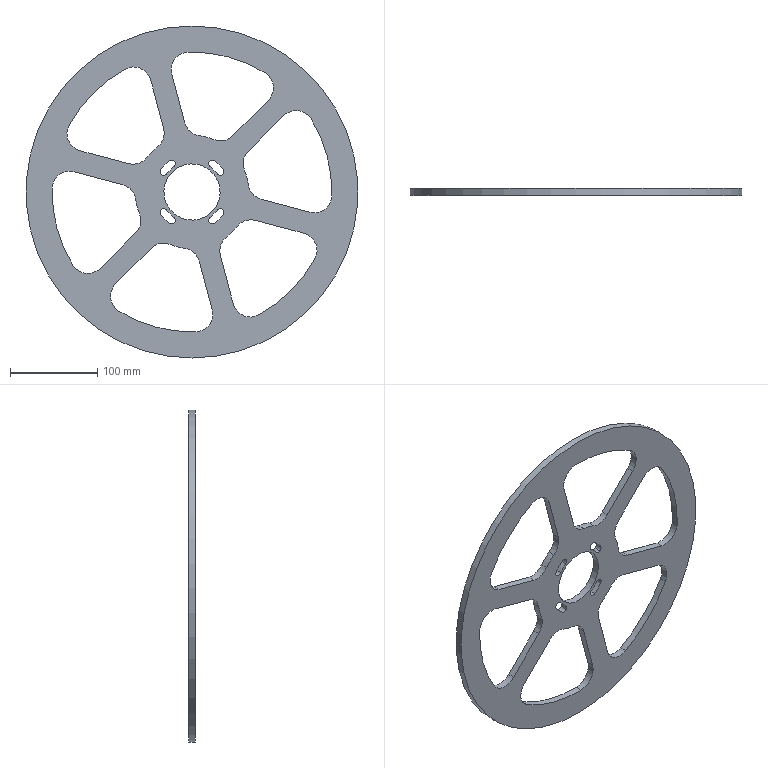Part | STEP file | 冲床-300配套压波_id1006_x_t | 1 solid | 76 faces | box 380 x 8 x 380 mm | volume 468890 mm3 | cylinder 62 | plane 14 | commonest cylinder face diameters 40 x24 8.7 x16 130 x6 320 x6 71.3 x4 88.7 x4